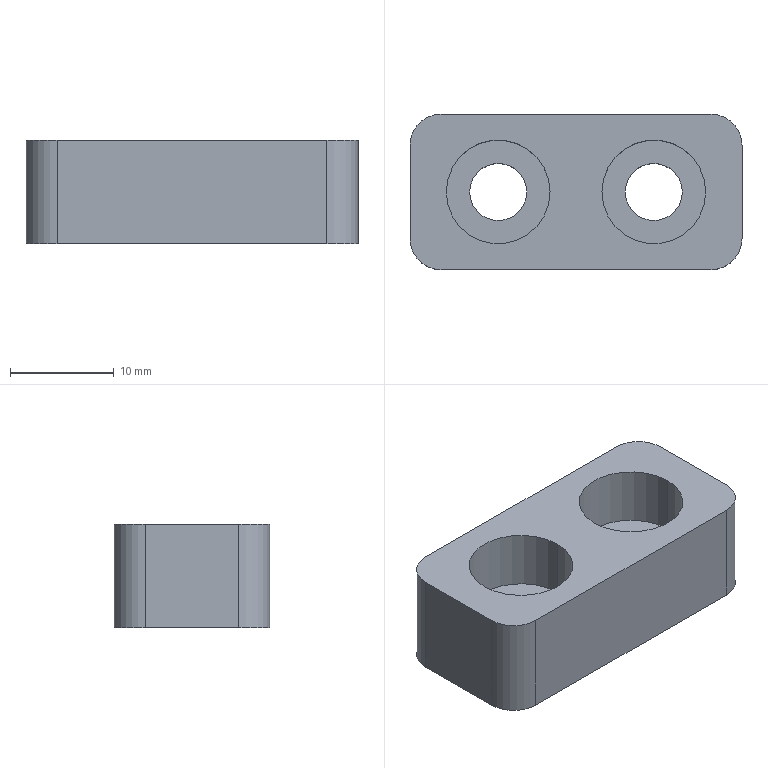Part | SolidWorks | features Extrusion 1, Fillet 1, HoleWzd 1 | 1 solid | 20 faces | box 32 x 15 x 10 mm | volume 3623 mm3 | cylinder 12 | plane 8 | commonest cylinder face diameters 5.5 x4 6 x4 10 x4
STEP:
#1=CARTESIAN_POINT('',(-12.5,0.,4.3));
#2=VERTEX_POINT('',#1);
#3=CARTESIAN_POINT('',(-2.5,0.,4.3));
#4=VERTEX_POINT('',#3);
#5=CARTESIAN_POINT('',(-7.5,0.,4.3));
#6=DIRECTION('',(0.,0.,1.));
#7=DIRECTION('',(1.,0.,0.));
#8=AXIS2_PLACEMENT_3D('',#5,#6,#7);
#9=CIRCLE('',#8,5.);
#10=EDGE_CURVE('',#2,#4,#9,.T.);
#11=ORIENTED_EDGE('',*,*,#10,.F.);
#12=CARTESIAN_POINT('',(-12.5,0.,10.));
#13=VERTEX_POINT('',#12);
#14=CARTESIAN_POINT('',(-12.5,0.,10.));
#15=DIRECTION('',(0.,0.,1.));
#16=VECTOR('',#15,1000.);
#17=LINE('',#14,#16);
#18=EDGE_CURVE('',#2,#13,#17,.T.);
#19=ORIENTED_EDGE('',*,*,#18,.T.);
#20=CARTESIAN_POINT('',(-2.5,0.,10.));
#21=VERTEX_POINT('',#20);
#22=CARTESIAN_POINT('',(-7.5,0.,10.));
#23=DIRECTION('',(0.,0.,1.));
#24=DIRECTION('',(1.,0.,0.));
#25=AXIS2_PLACEMENT_3D('',#22,#23,#24);
#26=CIRCLE('',#25,5.);
#27=EDGE_CURVE('',#13,#21,#26,.T.);
#28=ORIENTED_EDGE('',*,*,#27,.T.);
#29=CARTESIAN_POINT('',(-2.5,0.,10.));
#30=DIRECTION('',(0.,0.,1.));
#31=VECTOR('',#30,1000.);
#32=LINE('',#29,#31);
#33=EDGE_CURVE('',#4,#21,#32,.T.);
#34=ORIENTED_EDGE('',*,*,#33,.F.);
#35=EDGE_LOOP('',(#11,#19,#28,#34));
#36=FACE_OUTER_BOUND('',#35,.T.);
#37=CARTESIAN_POINT('',(-7.5,0.,10.));
#38=DIRECTION('',(0.,0.,1.));
#39=DIRECTION('',(1.,0.,0.));
#40=AXIS2_PLACEMENT_3D('',#37,#38,#39);
#41=CYLINDRICAL_SURFACE('',#40,5.);
#42=ADVANCED_FACE('',(#36),#41,.F.);
#43=CARTESIAN_POINT('',(-4.75,0.,0.));
#44=VERTEX_POINT('',#43);
#45=CARTESIAN_POINT('',(-10.25,0.,0.));
#46=VERTEX_POINT('',#45);
#47=CARTESIAN_POINT('',(-7.5,0.,0.));
#48=DIRECTION('',(0.,0.,-1.));
#49=DIRECTION('',(-1.,0.,0.));
#50=AXIS2_PLACEMENT_3D('',#47,#48,#49);
#51=CIRCLE('',#50,2.75);
#52=EDGE_CURVE('',#44,#46,#51,.T.);
#53=ORIENTED_EDGE('',*,*,#52,.T.);
#54=CARTESIAN_POINT('',(-10.25,0.,4.3));
#55=VERTEX_POINT('',#54);
#56=CARTESIAN_POINT('',(-10.25,0.,10.));
#57=DIRECTION('',(0.,0.,1.));
#58=VECTOR('',#57,1000.);
#59=LINE('',#56,#58);
#60=EDGE_CURVE('',#46,#55,#59,.T.);
#61=ORIENTED_EDGE('',*,*,#60,.T.);
#62=CARTESIAN_POINT('',(-4.75,0.,4.3));
#63=VERTEX_POINT('',#62);
#64=CARTESIAN_POINT('',(-7.5,0.,4.3));
#65=DIRECTION('',(0.,0.,1.));
#66=DIRECTION('',(1.,0.,0.));
#67=AXIS2_PLACEMENT_3D('',#64,#65,#66);
#68=CIRCLE('',#67,2.75);
#69=EDGE_CURVE('',#55,#63,#68,.T.);
#70=ORIENTED_EDGE('',*,*,#69,.T.);
#71=CARTESIAN_POINT('',(-4.75,0.,10.));
#72=DIRECTION('',(0.,0.,1.));
#73=VECTOR('',#72,1000.);
#74=LINE('',#71,#73);
#75=EDGE_CURVE('',#44,#63,#74,.T.);
#76=ORIENTED_EDGE('',*,*,#75,.F.);
#77=EDGE_LOOP('',(#53,#61,#70,#76));
#78=FACE_OUTER_BOUND('',#77,.T.);
#79=CARTESIAN_POINT('',(-7.5,0.,10.));
#80=DIRECTION('',(0.,0.,1.));
#81=DIRECTION('',(1.,0.,0.));
#82=AXIS2_PLACEMENT_3D('',#79,#80,#81);
#83=CYLINDRICAL_SURFACE('',#82,2.75);
#84=ADVANCED_FACE('',(#78),#83,.F.);
#85=CARTESIAN_POINT('',(2.5,0.,4.3));
#86=VERTEX_POINT('',#85);
#87=CARTESIAN_POINT('',(12.5,0.,4.3));
#88=VERTEX_POINT('',#87);
#89=CARTESIAN_POINT('',(7.5,0.,4.3));
#90=DIRECTION('',(0.,0.,1.));
#91=DIRECTION('',(1.,0.,0.));
#92=AXIS2_PLACEMENT_3D('',#89,#90,#91);
#93=CIRCLE('',#92,5.);
#94=EDGE_CURVE('',#86,#88,#93,.T.);
#95=ORIENTED_EDGE('',*,*,#94,.F.);
#96=CARTESIAN_POINT('',(2.5,0.,10.));
#97=VERTEX_POINT('',#96);
#98=CARTESIAN_POINT('',(2.5,0.,10.));
#99=DIRECTION('',(0.,0.,1.));
#100=VECTOR('',#99,1000.);
#101=LINE('',#98,#100);
#102=EDGE_CURVE('',#86,#97,#101,.T.);
#103=ORIENTED_EDGE('',*,*,#102,.T.);
#104=CARTESIAN_POINT('',(12.5,0.,10.));
#105=VERTEX_POINT('',#104);
#106=CARTESIAN_POINT('',(7.5,0.,10.));
#107=DIRECTION('',(0.,0.,1.));
#108=DIRECTION('',(1.,0.,0.));
#109=AXIS2_PLACEMENT_3D('',#106,#107,#108);
#110=CIRCLE('',#109,5.);
#111=EDGE_CURVE('',#97,#105,#110,.T.);
#112=ORIENTED_EDGE('',*,*,#111,.T.);
#113=CARTESIAN_POINT('',(12.5,0.,10.));
#114=DIRECTION('',(0.,0.,1.));
#115=VECTOR('',#114,1000.);
#116=LINE('',#113,#115);
#117=EDGE_CURVE('',#88,#105,#116,.T.);
#118=ORIENTED_EDGE('',*,*,#117,.F.);
#119=EDGE_LOOP('',(#95,#103,#112,#118));
#120=FACE_OUTER_BOUND('',#119,.T.);
#121=CARTESIAN_POINT('',(7.5,0.,10.));
#122=DIRECTION('',(0.,0.,1.));
#123=DIRECTION('',(1.,0.,0.));
#124=AXIS2_PLACEMENT_3D('',#121,#122,#123);
#125=CYLINDRICAL_SURFACE('',#124,5.);
#126=ADVANCED_FACE('',(#120),#125,.F.);
#127=CARTESIAN_POINT('',(10.25,0.,0.));
#128=VERTEX_POINT('',#127);
#129=CARTESIAN_POINT('',(4.75,0.,0.));
#130=VERTEX_POINT('',#129);
#131=CARTESIAN_POINT('',(7.5,0.,0.));
#132=DIRECTION('',(0.,0.,-1.));
#133=DIRECTION('',(-1.,0.,0.));
#134=AXIS2_PLACEMENT_3D('',#131,#132,#133);
#135=CIRCLE('',#134,2.75);
#136=EDGE_CURVE('',#128,#130,#135,.T.);
#137=ORIENTED_EDGE('',*,*,#136,.T.);
#138=CARTESIAN_POINT('',(4.75,0.,4.3));
#139=VERTEX_POINT('',#138);
#140=CARTESIAN_POINT('',(4.75,0.,10.));
#141=DIRECTION('',(0.,0.,1.));
#142=VECTOR('',#141,1000.);
#143=LINE('',#140,#142);
#144=EDGE_CURVE('',#130,#139,#143,.T.);
#145=ORIENTED_EDGE('',*,*,#144,.T.);
#146=CARTESIAN_POINT('',(10.25,0.,4.3));
#147=VERTEX_POINT('',#146);
#148=CARTESIAN_POINT('',(7.5,0.,4.3));
#149=DIRECTION('',(0.,0.,1.));
#150=DIRECTION('',(1.,0.,0.));
#151=AXIS2_PLACEMENT_3D('',#148,#149,#150);
#152=CIRCLE('',#151,2.75);
#153=EDGE_CURVE('',#139,#147,#152,.T.);
#154=ORIENTED_EDGE('',*,*,#153,.T.);
#155=CARTESIAN_POINT('',(10.25,0.,10.));
#156=DIRECTION('',(0.,0.,1.));
#157=VECTOR('',#156,1000.);
#158=LINE('',#155,#157);
#159=EDGE_CURVE('',#128,#147,#158,.T.);
#160=ORIENTED_EDGE('',*,*,#159,.F.);
#161=EDGE_LOOP('',(#137,#145,#154,#160));
#162=FACE_OUTER_BOUND('',#161,.T.);
#163=CARTESIAN_POINT('',(7.5,0.,10.));
#164=DIRECTION('',(0.,0.,1.));
#165=DIRECTION('',(1.,0.,0.));
#166=AXIS2_PLACEMENT_3D('',#163,#164,#165);
#167=CYLINDRICAL_SURFACE('',#166,2.75);
#168=ADVANCED_FACE('',(#162),#167,.F.);
#169=CARTESIAN_POINT('',(16.,-4.5,10.));
#170=VERTEX_POINT('',#169);
#171=CARTESIAN_POINT('',(16.,4.5,10.));
#172=VERTEX_POINT('',#171);
#173=CARTESIAN_POINT('',(16.,-7.5,10.));
#174=DIRECTION('',(0.,1.,0.));
#175=VECTOR('',#174,1000.);
#176=LINE('',#173,#175);
#177=EDGE_CURVE('',#170,#172,#176,.T.);
#178=ORIENTED_EDGE('',*,*,#177,.F.);
#179=CARTESIAN_POINT('',(16.,-4.5,0.));
#180=VERTEX_POINT('',#179);
#181=CARTESIAN_POINT('',(16.,-4.5,10.));
#182=DIRECTION('',(0.,0.,-1.));
#183=VECTOR('',#182,1000.);
#184=LINE('',#181,#183);
#185=EDGE_CURVE('',#170,#180,#184,.T.);
#186=ORIENTED_EDGE('',*,*,#185,.T.);
#187=CARTESIAN_POINT('',(16.,4.5,0.));
#188=VERTEX_POINT('',#187);
#189=CARTESIAN_POINT('',(16.,-7.5,0.));
#190=DIRECTION('',(0.,1.,0.));
#191=VECTOR('',#190,1000.);
#192=LINE('',#189,#191);
#193=EDGE_CURVE('',#180,#188,#192,.T.);
#194=ORIENTED_EDGE('',*,*,#193,.T.);
#195=CARTESIAN_POINT('',(16.,4.5,10.));
#196=DIRECTION('',(0.,0.,1.));
#197=VECTOR('',#196,1000.);
#198=LINE('',#195,#197);
#199=EDGE_CURVE('',#188,#172,#198,.T.);
#200=ORIENTED_EDGE('',*,*,#199,.T.);
#201=EDGE_LOOP('',(#178,#186,#194,#200));
#202=FACE_OUTER_BOUND('',#201,.T.);
#203=CARTESIAN_POINT('',(16.,-7.5,10.));
#204=DIRECTION('',(-1.,0.,0.));
#205=DIRECTION('',(0.,0.,1.));
#206=AXIS2_PLACEMENT_3D('',#203,#204,#205);
#207=PLANE('',#206);
#208=ADVANCED_FACE('',(#202),#207,.F.);
#209=CARTESIAN_POINT('',(13.,7.5,10.));
#210=VERTEX_POINT('',#209);
#211=CARTESIAN_POINT('',(-13.,7.5,10.));
#212=VERTEX_POINT('',#211);
#213=CARTESIAN_POINT('',(-16.,7.5,10.));
#214=DIRECTION('',(-1.,0.,0.));
#215=VECTOR('',#214,1000.);
#216=LINE('',#213,#215);
#217=EDGE_CURVE('',#210,#212,#216,.T.);
#218=ORIENTED_EDGE('',*,*,#217,.F.);
#219=CARTESIAN_POINT('',(13.,7.5,0.));
#220=VERTEX_POINT('',#219);
#221=CARTESIAN_POINT('',(13.,7.5,10.));
#222=DIRECTION('',(0.,0.,-1.));
#223=VECTOR('',#222,1000.);
#224=LINE('',#221,#223);
#225=EDGE_CURVE('',#210,#220,#224,.T.);
#226=ORIENTED_EDGE('',*,*,#225,.T.);
#227=CARTESIAN_POINT('',(-13.,7.5,0.));
#228=VERTEX_POINT('',#227);
#229=CARTESIAN_POINT('',(-16.,7.5,0.));
#230=DIRECTION('',(-1.,0.,0.));
#231=VECTOR('',#230,1000.);
#232=LINE('',#229,#231);
#233=EDGE_CURVE('',#220,#228,#232,.T.);
#234=ORIENTED_EDGE('',*,*,#233,.T.);
#235=CARTESIAN_POINT('',(-13.,7.5,10.));
#236=DIRECTION('',(0.,0.,1.));
#237=VECTOR('',#236,1000.);
#238=LINE('',#235,#237);
#239=EDGE_CURVE('',#228,#212,#238,.T.);
#240=ORIENTED_EDGE('',*,*,#239,.T.);
#241=EDGE_LOOP('',(#218,#226,#234,#240));
#242=FACE_OUTER_BOUND('',#241,.T.);
#243=CARTESIAN_POINT('',(-16.,7.5,10.));
#244=DIRECTION('',(0.,-1.,0.));
#245=DIRECTION('',(0.,0.,-1.));
#246=AXIS2_PLACEMENT_3D('',#243,#244,#245);
#247=PLANE('',#246);
#248=ADVANCED_FACE('',(#242),#247,.F.);
#249=CARTESIAN_POINT('',(-16.,4.5,0.));
#250=VERTEX_POINT('',#249);
#251=CARTESIAN_POINT('',(-16.,-4.5,0.));
#252=VERTEX_POINT('',#251);
#253=CARTESIAN_POINT('',(-16.,-7.5,0.));
#254=DIRECTION('',(0.,-1.,0.));
#255=VECTOR('',#254,1000.);
#256=LINE('',#253,#255);
#257=EDGE_CURVE('',#250,#252,#256,.T.);
#258=ORIENTED_EDGE('',*,*,#257,.T.);
#259=CARTESIAN_POINT('',(-16.,-4.5,10.));
#260=VERTEX_POINT('',#259);
#261=CARTESIAN_POINT('',(-16.,-4.5,10.));
#262=DIRECTION('',(0.,0.,1.));
#263=VECTOR('',#262,1000.);
#264=LINE('',#261,#263);
#265=EDGE_CURVE('',#252,#260,#264,.T.);
#266=ORIENTED_EDGE('',*,*,#265,.T.);
#267=CARTESIAN_POINT('',(-16.,4.5,10.));
#268=VERTEX_POINT('',#267);
#269=CARTESIAN_POINT('',(-16.,-7.5,10.));
#270=DIRECTION('',(0.,-1.,0.));
#271=VECTOR('',#270,1000.);
#272=LINE('',#269,#271);
#273=EDGE_CURVE('',#268,#260,#272,.T.);
#274=ORIENTED_EDGE('',*,*,#273,.F.);
#275=CARTESIAN_POINT('',(-16.,4.5,10.));
#276=DIRECTION('',(0.,0.,-1.));
#277=VECTOR('',#276,1000.);
#278=LINE('',#275,#277);
#279=EDGE_CURVE('',#268,#250,#278,.T.);
#280=ORIENTED_EDGE('',*,*,#279,.T.);
#281=EDGE_LOOP('',(#258,#266,#274,#280));
#282=FACE_OUTER_BOUND('',#281,.T.);
#283=CARTESIAN_POINT('',(-16.,-7.5,10.));
#284=DIRECTION('',(1.,0.,0.));
#285=DIRECTION('',(0.,0.,-1.));
#286=AXIS2_PLACEMENT_3D('',#283,#284,#285);
#287=PLANE('',#286);
#288=ADVANCED_FACE('',(#282),#287,.F.);
#289=CARTESIAN_POINT('',(-13.,-7.5,0.));
#290=VERTEX_POINT('',#289);
#291=CARTESIAN_POINT('',(13.,-7.5,0.));
#292=VERTEX_POINT('',#291);
#293=CARTESIAN_POINT('',(-16.,-7.5,0.));
#294=DIRECTION('',(1.,0.,0.));
#295=VECTOR('',#294,1000.);
#296=LINE('',#293,#295);
#297=EDGE_CURVE('',#290,#292,#296,.T.);
#298=ORIENTED_EDGE('',*,*,#297,.T.);
#299=CARTESIAN_POINT('',(13.,-7.5,10.));
#300=VERTEX_POINT('',#299);
#301=CARTESIAN_POINT('',(13.,-7.5,10.));
#302=DIRECTION('',(0.,0.,1.));
#303=VECTOR('',#302,1000.);
#304=LINE('',#301,#303);
#305=EDGE_CURVE('',#292,#300,#304,.T.);
#306=ORIENTED_EDGE('',*,*,#305,.T.);
#307=CARTESIAN_POINT('',(-13.,-7.5,10.));
#308=VERTEX_POINT('',#307);
#309=CARTESIAN_POINT('',(-16.,-7.5,10.));
#310=DIRECTION('',(1.,0.,0.));
#311=VECTOR('',#310,1000.);
#312=LINE('',#309,#311);
#313=EDGE_CURVE('',#308,#300,#312,.T.);
#314=ORIENTED_EDGE('',*,*,#313,.F.);
#315=CARTESIAN_POINT('',(-13.,-7.5,10.));
#316=DIRECTION('',(0.,0.,-1.));
#317=VECTOR('',#316,1000.);
#318=LINE('',#315,#317);
#319=EDGE_CURVE('',#308,#290,#318,.T.);
#320=ORIENTED_EDGE('',*,*,#319,.T.);
#321=EDGE_LOOP('',(#298,#306,#314,#320));
#322=FACE_OUTER_BOUND('',#321,.T.);
#323=CARTESIAN_POINT('',(-16.,-7.5,10.));
#324=DIRECTION('',(0.,1.,0.));
#325=DIRECTION('',(0.,0.,1.));
#326=AXIS2_PLACEMENT_3D('',#323,#324,#325);
#327=PLANE('',#326);
#328=ADVANCED_FACE('',(#322),#327,.F.);
#329=CARTESIAN_POINT('',(-7.5,0.,10.));
#330=DIRECTION('',(0.,0.,1.));
#331=DIRECTION('',(1.,0.,0.));
#332=AXIS2_PLACEMENT_3D('',#329,#330,#331);
#333=CIRCLE('',#332,5.);
#334=EDGE_CURVE('',#21,#13,#333,.T.);
#335=ORIENTED_EDGE('',*,*,#334,.F.);
#336=ORIENTED_EDGE('',*,*,#27,.F.);
#337=EDGE_LOOP('',(#335,#336));
#338=FACE_BOUND('',#337,.T.);
#339=CARTESIAN_POINT('',(7.5,0.,10.));
#340=DIRECTION('',(0.,0.,1.));
#341=DIRECTION('',(1.,0.,0.));
#342=AXIS2_PLACEMENT_3D('',#339,#340,#341);
#343=CIRCLE('',#342,5.);
#344=EDGE_CURVE('',#105,#97,#343,.T.);
#345=ORIENTED_EDGE('',*,*,#344,.F.);
#346=ORIENTED_EDGE('',*,*,#111,.F.);
#347=EDGE_LOOP('',(#345,#346));
#348=FACE_BOUND('',#347,.T.);
#349=ORIENTED_EDGE('',*,*,#313,.T.);
#350=CARTESIAN_POINT('',(13.,-4.5,10.));
#351=DIRECTION('',(0.,0.,1.));
#352=DIRECTION('',(-1.,0.,0.));
#353=AXIS2_PLACEMENT_3D('',#350,#351,#352);
#354=CIRCLE('',#353,3.);
#355=EDGE_CURVE('',#300,#170,#354,.T.);
#356=ORIENTED_EDGE('',*,*,#355,.T.);
#357=ORIENTED_EDGE('',*,*,#177,.T.);
#358=CARTESIAN_POINT('',(13.,4.5,10.));
#359=DIRECTION('',(0.,0.,1.));
#360=DIRECTION('',(-1.,0.,0.));
#361=AXIS2_PLACEMENT_3D('',#358,#359,#360);
#362=CIRCLE('',#361,3.);
#363=EDGE_CURVE('',#172,#210,#362,.T.);
#364=ORIENTED_EDGE('',*,*,#363,.T.);
#365=ORIENTED_EDGE('',*,*,#217,.T.);
#366=CARTESIAN_POINT('',(-13.,4.5,10.));
#367=DIRECTION('',(0.,0.,1.));
#368=DIRECTION('',(-1.,0.,0.));
#369=AXIS2_PLACEMENT_3D('',#366,#367,#368);
#370=CIRCLE('',#369,3.);
#371=EDGE_CURVE('',#212,#268,#370,.T.);
#372=ORIENTED_EDGE('',*,*,#371,.T.);
#373=ORIENTED_EDGE('',*,*,#273,.T.);
#374=CARTESIAN_POINT('',(-13.,-4.5,10.));
#375=DIRECTION('',(0.,0.,1.));
#376=DIRECTION('',(-1.,0.,0.));
#377=AXIS2_PLACEMENT_3D('',#374,#375,#376);
#378=CIRCLE('',#377,3.);
#379=EDGE_CURVE('',#260,#308,#378,.T.);
#380=ORIENTED_EDGE('',*,*,#379,.T.);
#381=EDGE_LOOP('',(#349,#356,#357,#364,#365,#372,#373,#380));
#382=FACE_OUTER_BOUND('',#381,.T.);
#383=CARTESIAN_POINT('',(0.,0.,10.));
#384=DIRECTION('',(0.,0.,-1.));
#385=DIRECTION('',(-1.,0.,0.));
#386=AXIS2_PLACEMENT_3D('',#383,#384,#385);
#387=PLANE('',#386);
#388=ADVANCED_FACE('',(#338,#348,#382),#387,.F.);
#389=ORIENTED_EDGE('',*,*,#52,.F.);
#390=CARTESIAN_POINT('',(-7.5,0.,0.));
#391=DIRECTION('',(0.,0.,-1.));
#392=DIRECTION('',(-1.,0.,0.));
#393=AXIS2_PLACEMENT_3D('',#390,#391,#392);
#394=CIRCLE('',#393,2.75);
#395=EDGE_CURVE('',#46,#44,#394,.T.);
#396=ORIENTED_EDGE('',*,*,#395,.F.);
#397=EDGE_LOOP('',(#389,#396));
#398=FACE_BOUND('',#397,.T.);
#399=ORIENTED_EDGE('',*,*,#136,.F.);
#400=CARTESIAN_POINT('',(7.5,0.,0.));
#401=DIRECTION('',(0.,0.,-1.));
#402=DIRECTION('',(-1.,0.,0.));
#403=AXIS2_PLACEMENT_3D('',#400,#401,#402);
#404=CIRCLE('',#403,2.75);
#405=EDGE_CURVE('',#130,#128,#404,.T.);
#406=ORIENTED_EDGE('',*,*,#405,.F.);
#407=EDGE_LOOP('',(#399,#406));
#408=FACE_BOUND('',#407,.T.);
#409=ORIENTED_EDGE('',*,*,#193,.F.);
#410=CARTESIAN_POINT('',(13.,-4.5,0.));
#411=DIRECTION('',(0.,0.,-1.));
#412=DIRECTION('',(-1.,0.,0.));
#413=AXIS2_PLACEMENT_3D('',#410,#411,#412);
#414=CIRCLE('',#413,3.);
#415=EDGE_CURVE('',#180,#292,#414,.T.);
#416=ORIENTED_EDGE('',*,*,#415,.T.);
#417=ORIENTED_EDGE('',*,*,#297,.F.);
#418=CARTESIAN_POINT('',(-13.,-4.5,0.));
#419=DIRECTION('',(0.,0.,-1.));
#420=DIRECTION('',(-1.,0.,0.));
#421=AXIS2_PLACEMENT_3D('',#418,#419,#420);
#422=CIRCLE('',#421,3.);
#423=EDGE_CURVE('',#290,#252,#422,.T.);
#424=ORIENTED_EDGE('',*,*,#423,.T.);
#425=ORIENTED_EDGE('',*,*,#257,.F.);
#426=CARTESIAN_POINT('',(-13.,4.5,0.));
#427=DIRECTION('',(0.,0.,-1.));
#428=DIRECTION('',(-1.,0.,0.));
#429=AXIS2_PLACEMENT_3D('',#426,#427,#428);
#430=CIRCLE('',#429,3.);
#431=EDGE_CURVE('',#250,#228,#430,.T.);
#432=ORIENTED_EDGE('',*,*,#431,.T.);
#433=ORIENTED_EDGE('',*,*,#233,.F.);
#434=CARTESIAN_POINT('',(13.,4.5,0.));
#435=DIRECTION('',(0.,0.,-1.));
#436=DIRECTION('',(-1.,0.,0.));
#437=AXIS2_PLACEMENT_3D('',#434,#435,#436);
#438=CIRCLE('',#437,3.);
#439=EDGE_CURVE('',#220,#188,#438,.T.);
#440=ORIENTED_EDGE('',*,*,#439,.T.);
#441=EDGE_LOOP('',(#409,#416,#417,#424,#425,#432,#433,#440));
#442=FACE_OUTER_BOUND('',#441,.T.);
#443=CARTESIAN_POINT('',(0.,0.,0.));
#444=DIRECTION('',(0.,0.,-1.));
#445=DIRECTION('',(-1.,0.,0.));
#446=AXIS2_PLACEMENT_3D('',#443,#444,#445);
#447=PLANE('',#446);
#448=ADVANCED_FACE('',(#398,#408,#442),#447,.T.);
#449=ORIENTED_EDGE('',*,*,#144,.F.);
#450=ORIENTED_EDGE('',*,*,#405,.T.);
#451=ORIENTED_EDGE('',*,*,#159,.T.);
#452=CARTESIAN_POINT('',(7.5,0.,4.3));
#453=DIRECTION('',(0.,0.,1.));
#454=DIRECTION('',(1.,0.,0.));
#455=AXIS2_PLACEMENT_3D('',#452,#453,#454);
#456=CIRCLE('',#455,2.75);
#457=EDGE_CURVE('',#147,#139,#456,.T.);
#458=ORIENTED_EDGE('',*,*,#457,.T.);
#459=EDGE_LOOP('',(#449,#450,#451,#458));
#460=FACE_OUTER_BOUND('',#459,.T.);
#461=CARTESIAN_POINT('',(7.5,0.,10.));
#462=DIRECTION('',(0.,0.,1.));
#463=DIRECTION('',(1.,0.,0.));
#464=AXIS2_PLACEMENT_3D('',#461,#462,#463);
#465=CYLINDRICAL_SURFACE('',#464,2.75);
#466=ADVANCED_FACE('',(#460),#465,.F.);
#467=ORIENTED_EDGE('',*,*,#457,.F.);
#468=ORIENTED_EDGE('',*,*,#153,.F.);
#469=EDGE_LOOP('',(#467,#468));
#470=FACE_BOUND('',#469,.T.);
#471=CARTESIAN_POINT('',(7.5,0.,4.3));
#472=DIRECTION('',(0.,0.,1.));
#473=DIRECTION('',(1.,0.,0.));
#474=AXIS2_PLACEMENT_3D('',#471,#472,#473);
#475=CIRCLE('',#474,5.);
#476=EDGE_CURVE('',#88,#86,#475,.T.);
#477=ORIENTED_EDGE('',*,*,#476,.T.);
#478=ORIENTED_EDGE('',*,*,#94,.T.);
#479=EDGE_LOOP('',(#477,#478));
#480=FACE_OUTER_BOUND('',#479,.T.);
#481=CARTESIAN_POINT('',(10.25,0.,4.3));
#482=DIRECTION('',(0.,0.,-1.));
#483=DIRECTION('',(-1.,0.,0.));
#484=AXIS2_PLACEMENT_3D('',#481,#482,#483);
#485=PLANE('',#484);
#486=ADVANCED_FACE('',(#470,#480),#485,.F.);
#487=ORIENTED_EDGE('',*,*,#102,.F.);
#488=ORIENTED_EDGE('',*,*,#476,.F.);
#489=ORIENTED_EDGE('',*,*,#117,.T.);
#490=ORIENTED_EDGE('',*,*,#344,.T.);
#491=EDGE_LOOP('',(#487,#488,#489,#490));
#492=FACE_OUTER_BOUND('',#491,.T.);
#493=CARTESIAN_POINT('',(7.5,0.,10.));
#494=DIRECTION('',(0.,0.,1.));
#495=DIRECTION('',(1.,0.,0.));
#496=AXIS2_PLACEMENT_3D('',#493,#494,#495);
#497=CYLINDRICAL_SURFACE('',#496,5.);
#498=ADVANCED_FACE('',(#492),#497,.F.);
#499=ORIENTED_EDGE('',*,*,#60,.F.);
#500=ORIENTED_EDGE('',*,*,#395,.T.);
#501=ORIENTED_EDGE('',*,*,#75,.T.);
#502=CARTESIAN_POINT('',(-7.5,0.,4.3));
#503=DIRECTION('',(0.,0.,1.));
#504=DIRECTION('',(1.,0.,0.));
#505=AXIS2_PLACEMENT_3D('',#502,#503,#504);
#506=CIRCLE('',#505,2.75);
#507=EDGE_CURVE('',#63,#55,#506,.T.);
#508=ORIENTED_EDGE('',*,*,#507,.T.);
#509=EDGE_LOOP('',(#499,#500,#501,#508));
#510=FACE_OUTER_BOUND('',#509,.T.);
#511=CARTESIAN_POINT('',(-7.5,0.,10.));
#512=DIRECTION('',(0.,0.,1.));
#513=DIRECTION('',(1.,0.,0.));
#514=AXIS2_PLACEMENT_3D('',#511,#512,#513);
#515=CYLINDRICAL_SURFACE('',#514,2.75);
#516=ADVANCED_FACE('',(#510),#515,.F.);
#517=ORIENTED_EDGE('',*,*,#507,.F.);
#518=ORIENTED_EDGE('',*,*,#69,.F.);
#519=EDGE_LOOP('',(#517,#518));
#520=FACE_BOUND('',#519,.T.);
#521=CARTESIAN_POINT('',(-7.5,0.,4.3));
#522=DIRECTION('',(0.,0.,1.));
#523=DIRECTION('',(1.,0.,0.));
#524=AXIS2_PLACEMENT_3D('',#521,#522,#523);
#525=CIRCLE('',#524,5.);
#526=EDGE_CURVE('',#4,#2,#525,.T.);
#527=ORIENTED_EDGE('',*,*,#526,.T.);
#528=ORIENTED_EDGE('',*,*,#10,.T.);
#529=EDGE_LOOP('',(#527,#528));
#530=FACE_OUTER_BOUND('',#529,.T.);
#531=CARTESIAN_POINT('',(-4.75,0.,4.3));
#532=DIRECTION('',(0.,0.,-1.));
#533=DIRECTION('',(-1.,0.,0.));
#534=AXIS2_PLACEMENT_3D('',#531,#532,#533);
#535=PLANE('',#534);
#536=ADVANCED_FACE('',(#520,#530),#535,.F.);
#537=ORIENTED_EDGE('',*,*,#18,.F.);
#538=ORIENTED_EDGE('',*,*,#526,.F.);
#539=ORIENTED_EDGE('',*,*,#33,.T.);
#540=ORIENTED_EDGE('',*,*,#334,.T.);
#541=EDGE_LOOP('',(#537,#538,#539,#540));
#542=FACE_OUTER_BOUND('',#541,.T.);
#543=CARTESIAN_POINT('',(-7.5,0.,10.));
#544=DIRECTION('',(0.,0.,1.));
#545=DIRECTION('',(1.,0.,0.));
#546=AXIS2_PLACEMENT_3D('',#543,#544,#545);
#547=CYLINDRICAL_SURFACE('',#546,5.);
#548=ADVANCED_FACE('',(#542),#547,.F.);
#549=ORIENTED_EDGE('',*,*,#355,.F.);
#550=ORIENTED_EDGE('',*,*,#305,.F.);
#551=ORIENTED_EDGE('',*,*,#415,.F.);
#552=ORIENTED_EDGE('',*,*,#185,.F.);
#553=EDGE_LOOP('',(#549,#550,#551,#552));
#554=FACE_OUTER_BOUND('',#553,.T.);
#555=CARTESIAN_POINT('',(13.,-4.5,10.));
#556=DIRECTION('',(0.,0.,-1.));
#557=DIRECTION('',(-1.,0.,0.));
#558=AXIS2_PLACEMENT_3D('',#555,#556,#557);
#559=CYLINDRICAL_SURFACE('',#558,3.);
#560=ADVANCED_FACE('',(#554),#559,.T.);
#561=ORIENTED_EDGE('',*,*,#363,.F.);
#562=ORIENTED_EDGE('',*,*,#199,.F.);
#563=ORIENTED_EDGE('',*,*,#439,.F.);
#564=ORIENTED_EDGE('',*,*,#225,.F.);
#565=EDGE_LOOP('',(#561,#562,#563,#564));
#566=FACE_OUTER_BOUND('',#565,.T.);
#567=CARTESIAN_POINT('',(13.,4.5,10.));
#568=DIRECTION('',(0.,0.,-1.));
#569=DIRECTION('',(-1.,0.,0.));
#570=AXIS2_PLACEMENT_3D('',#567,#568,#569);
#571=CYLINDRICAL_SURFACE('',#570,3.);
#572=ADVANCED_FACE('',(#566),#571,.T.);
#573=ORIENTED_EDGE('',*,*,#379,.F.);
#574=ORIENTED_EDGE('',*,*,#265,.F.);
#575=ORIENTED_EDGE('',*,*,#423,.F.);
#576=ORIENTED_EDGE('',*,*,#319,.F.);
#577=EDGE_LOOP('',(#573,#574,#575,#576));
#578=FACE_OUTER_BOUND('',#577,.T.);
#579=CARTESIAN_POINT('',(-13.,-4.5,10.));
#580=DIRECTION('',(0.,0.,-1.));
#581=DIRECTION('',(-1.,0.,0.));
#582=AXIS2_PLACEMENT_3D('',#579,#580,#581);
#583=CYLINDRICAL_SURFACE('',#582,3.);
#584=ADVANCED_FACE('',(#578),#583,.T.);
#585=ORIENTED_EDGE('',*,*,#371,.F.);
#586=ORIENTED_EDGE('',*,*,#239,.F.);
#587=ORIENTED_EDGE('',*,*,#431,.F.);
#588=ORIENTED_EDGE('',*,*,#279,.F.);
#589=EDGE_LOOP('',(#585,#586,#587,#588));
#590=FACE_OUTER_BOUND('',#589,.T.);
#591=CARTESIAN_POINT('',(-13.,4.5,10.));
#592=DIRECTION('',(0.,0.,-1.));
#593=DIRECTION('',(-1.,0.,0.));
#594=AXIS2_PLACEMENT_3D('',#591,#592,#593);
#595=CYLINDRICAL_SURFACE('',#594,3.);
#596=ADVANCED_FACE('',(#590),#595,.T.);
#597=CLOSED_SHELL('',(#42,#84,#126,#168,#208,#248,#288,#328,#388,#448,#466,#486,#498,#516,#536,#548,#560,#572,#584,#596));
#598=MANIFOLD_SOLID_BREP('',#597);
#599=CARTESIAN_POINT('',(0.,0.,0.));
#600=DIRECTION('',(0.,0.,1.));
#601=DIRECTION('',(1.,0.,0.));
#602=AXIS2_PLACEMENT_3D('',#599,#600,#601);
#603=(LENGTH_UNIT()NAMED_UNIT(*)SI_UNIT(.MILLI.,.METRE.));
#604=UNCERTAINTY_MEASURE_WITH_UNIT(LENGTH_MEASURE(0.00001),#603,'','');
#605=(NAMED_UNIT(*)PLANE_ANGLE_UNIT()SI_UNIT($,.RADIAN.));
#606=(NAMED_UNIT(*)SI_UNIT($,.STERADIAN.)SOLID_ANGLE_UNIT());
#607=(GEOMETRIC_REPRESENTATION_CONTEXT(3)GLOBAL_UNCERTAINTY_ASSIGNED_CONTEXT((#604))GLOBAL_UNIT_ASSIGNED_CONTEXT((#603,#605,#606))REPRESENTATION_CONTEXT('',''));
#608=ADVANCED_BREP_SHAPE_REPRESENTATION('',(#598,#602),#607);